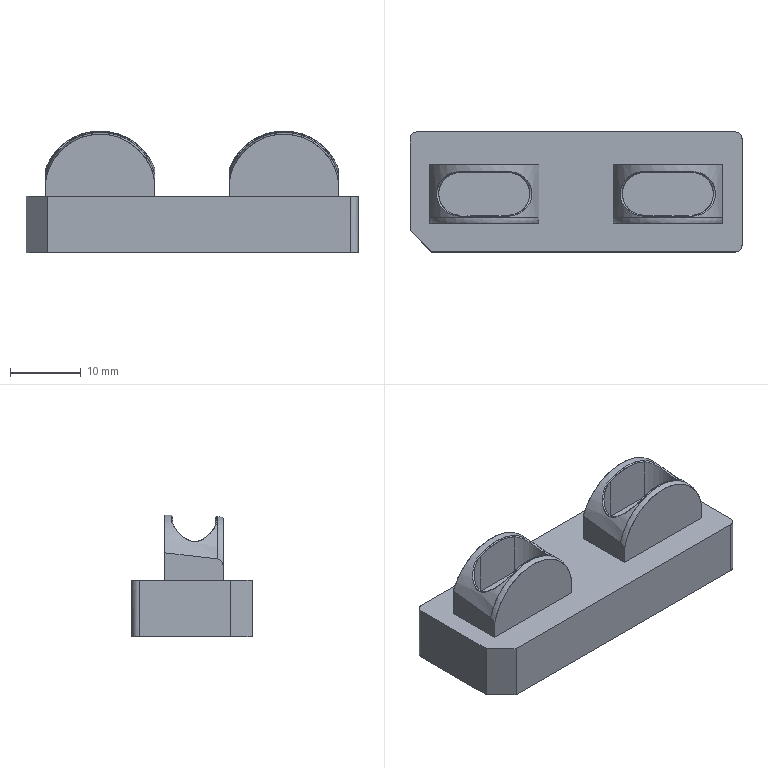NC program | PowerMill | posted with a generic post | part box 47 x 17 x 17.251 mm
Lines 19120 to 19835 of 158620:
N19217 M6
N19218 S22000 M03
N19219 G00 G90 X0.0 Y0.0
N19220 G43 Z10.798 H22
N19221
N19222 G05 P10000 R8
N19223 X21.9085 Y-5.0226
N19224 Z-6.8806
N19225 G01 Z-8.0806 F1200.0
N19226 X21.8959 Y-5.0352 Z-8.0493 F2000.0
N19227 X21.776 Y-5.0985 Z-7.6809
N19228 X21.7984 Y-5.0762 Z-7.7191
N19229 X21.8192 Y-5.0553 Z-7.7588
N19230 X21.8415 Y-5.033 Z-7.8048
N19231 X21.8681 Y-5.0064 Z-7.8637
N19232 X21.9 Y-4.9745 Z-7.9399
N19233 X21.9227 Y-4.9518 Z-7.9972
N19234 X21.9402 Y-4.9343 Z-8.0436
N19235 X21.9562 Y-4.9183 Z-8.0879
N19236 X21.9696 Y-4.9049 Z-8.1266
N19237 X22.0098 Y-4.8082 Z-8.1378
N19238 X22.0056 Y-4.8124 Z-8.1246
N19239 X21.9907 Y-4.8273 Z-8.0793
N19240 X21.9738 Y-4.8442 Z-8.0302
N19241 X21.9534 Y-4.8645 Z-7.9735
N19242 X21.9284 Y-4.8895 Z-7.9073
N19243 X21.8968 Y-4.9212 Z-7.8277
N19244 X21.8585 Y-4.9595 Z-7.7376
N19245 X21.8256 Y-4.9924 Z-7.6656
N19246 X21.7966 Y-5.0214 Z-7.6064
N19247 X21.7704 Y-5.0476 Z-7.5566
N19248 X21.7463 Y-5.0716 Z-7.5144
N19249 X21.7232 Y-5.0948 Z-7.4771
N19250 X21.6984 Y-5.1195 Z-7.4417
N19251 X21.6389 Y-5.1224 Z-7.2494
N19252 X21.6726 Y-5.0888 Z-7.2948
N19253 X21.7044 Y-5.0569 Z-7.3426
N19254 X21.7356 Y-5.0258 Z-7.3947
N19255 X21.7683 Y-4.9931 Z-7.4549
N19256 X21.8037 Y-4.9577 Z-7.5263
N19257 X21.8383 Y-4.923 Z-7.6003
N19258 X21.8719 Y-4.8895 Z-7.6747
N19259 X21.9129 Y-4.8485 Z-7.7716
N19260 X21.9529 Y-4.8085 Z-7.8737
N19261 X21.9897 Y-4.7717 Z-7.9758
N19262 X22.0228 Y-4.7385 Z-8.0758
N19263 X22.037 Y-4.7243 Z-8.1216
N19264 X22.0609 Y-4.6439 Z-8.1063
N19265 X22.0439 Y-4.6609 Z-8.0497
N19266 X22.0116 Y-4.6932 Z-7.9496
N19267 X21.9745 Y-4.7303 Z-7.8438
N19268 X21.9358 Y-4.769 Z-7.7414
N19269 X21.897 Y-4.8078 Z-7.6459
N19270 X21.8571 Y-4.8477 Z-7.5539
N19271 X21.8136 Y-4.8912 Z-7.46
N19272 X21.7702 Y-4.9346 Z-7.3732
N19273 X21.7462 Y-4.9586 Z-7.3279
N19274 X21.7218 Y-4.983 Z-7.2829
N19275 X21.6969 Y-5.0079 Z-7.2385
N19276 X21.6678 Y-5.037 Z-7.1906
N19277 X21.6402 Y-5.0646 Z-7.1495
N19278 X21.6114 Y-5.0934 Z-7.1105
N19279 X21.5813 Y-5.1235 Z-7.0731
N19280 X21.5247 Y-5.1236 Z-6.9091
N19281 X21.5585 Y-5.0898 Z-6.9483
N19282 X21.5926 Y-5.0557 Z-6.9927
N19283 X21.6276 Y-5.0206 Z-7.0437
N19284 X21.6648 Y-4.9834 Z-7.1031
N19285 X21.7063 Y-4.9419 Z-7.175
N19286 X21.7545 Y-4.8937 Z-7.263
N19287 X21.7917 Y-4.8565 Z-7.3347
N19288 X21.8271 Y-4.8211 Z-7.4081
N19289 X21.8612 Y-4.7871 Z-7.4829
N19290 X21.8979 Y-4.7504 Z-7.5683
N19291 X21.9396 Y-4.7086 Z-7.6715
N19292 X21.978 Y-4.6703 Z-7.7726
N19293 X22.0087 Y-4.6396 Z-7.8588
N19294 X22.0355 Y-4.6127 Z-7.9393
N19295 X22.0608 Y-4.5874 Z-8.0207
N19296 X22.0805 Y-4.5677 Z-8.0902
N19297 X22.0966 Y-4.495 Z-8.0754
N19298 X22.0885 Y-4.5031 Z-8.0396
N19299 X22.0746 Y-4.5171 Z-7.9886
N19300 X22.0622 Y-4.5295 Z-7.9464
N19301 X22.0417 Y-4.55 Z-7.8811
N19302 X22.0201 Y-4.5715 Z-7.8166
N19303 X21.9979 Y-4.5938 Z-7.7525
N19304 X21.9748 Y-4.6169 Z-7.6889
N19305 X21.9338 Y-4.6579 Z-7.5822
N19306 X21.8888 Y-4.7029 Z-7.4729
N19307 X21.8438 Y-4.7478 Z-7.3709
N19308 X21.8 Y-4.7917 Z-7.2781
N19309 X21.7575 Y-4.8342 Z-7.1942
N19310 X21.7077 Y-4.884 Z-7.1017
N19311 X21.662 Y-4.9296 Z-7.0222
N19312 X21.6188 Y-4.9729 Z-6.9524
N19313 X21.5758 Y-5.0159 Z-6.8886
N19314 X21.5376 Y-5.054 Z-6.8365
N19315 X21.5021 Y-5.0896 Z-6.7927
N19316 X21.4679 Y-5.1237 Z-6.7551
N19317 X21.4123 Y-5.1228 Z-6.6101
N19318 X21.4412 Y-5.0939 Z-6.6386
N19319 X21.4705 Y-5.0646 Z-6.6715
N19320 X21.503 Y-5.0321 Z-6.712
N19321 X21.5399 Y-4.9952 Z-6.7625
N19322 X21.5829 Y-4.9522 Z-6.8263
N19323 X21.6176 Y-4.9175 Z-6.8809
N19324 X21.6453 Y-4.8898 Z-6.9261
N19325 X21.6701 Y-4.865 Z-6.9673
N19326 X21.7179 Y-4.8172 Z-7.0514
N19327 X21.7653 Y-4.7698 Z-7.141
N19328 X21.8126 Y-4.7225 Z-7.237
N19329 X21.86 Y-4.6751 Z-7.3399
N19330 X21.9079 Y-4.6272 Z-7.451
N19331 X21.9454 Y-4.5897 Z-7.5432
N19332 X21.966 Y-4.5691 Z-7.5959
N19333 X21.9856 Y-4.5495 Z-7.6494
N19334 X22.0042 Y-4.5309 Z-7.7035
N19335 X22.0229 Y-4.5122 Z-7.7576
N19336 X22.0415 Y-4.4936 Z-7.8119
N19337 X22.0671 Y-4.468 Z-7.8937
N19338 X22.0889 Y-4.4462 Z-7.9723
N19339 X22.1072 Y-4.4279 Z-8.0482
N19340 X22.1079 Y-4.4272 Z-8.0517
N19341 X22.1147 Y-4.3639 Z-8.0167
N19342 X22.1118 Y-4.3667 Z-8.001
N19343 X22.1005 Y-4.378 Z-7.9478
N19344 X22.0853 Y-4.3933 Z-7.8892
N19345 X22.0647 Y-4.4138 Z-7.8208
N19346 X22.0341 Y-4.4445 Z-7.7261
N19347 X22.0009 Y-4.4776 Z-7.6281
N19348 X21.9614 Y-4.5171 Z-7.5202
N19349 X21.9196 Y-4.5589 Z-7.4145
N19350 X21.8759 Y-4.6026 Z-7.3121
N19351 X21.8305 Y-4.648 Z-7.2124
N19352 X21.7795 Y-4.699 Z-7.1066
N19353 X21.7297 Y-4.7488 Z-7.0096
N19354 X21.6804 Y-4.7981 Z-6.92
N19355 X21.6314 Y-4.8471 Z-6.8369
N19356 X21.5935 Y-4.885 Z-6.7766
N19357 X21.551 Y-4.9275 Z-6.7113
N19358 X21.5052 Y-4.9734 Z-6.6447
N19359 X21.4639 Y-5.0146 Z-6.5893
N19360 X21.4263 Y-5.0522 Z-6.5432
N19361 X21.3912 Y-5.0873 Z-6.5045
N19362 X21.3575 Y-5.121 Z-6.4717
N19363 X21.3027 Y-5.1193 Z-6.3407
N19364 X21.34 Y-5.0819 Z-6.3758
N19365 X21.3783 Y-5.0437 Z-6.4163
N19366 X21.4183 Y-5.0037 Z-6.4635
N19367 X21.4614 Y-4.9605 Z-6.5193
N19368 X21.4959 Y-4.9261 Z-6.5669
N19369 X21.5507 Y-4.8713 Z-6.647
N19370 X21.6048 Y-4.8172 Z-6.7317
N19371 X21.6583 Y-4.7637 Z-6.8213
N19372 X21.7112 Y-4.7107 Z-6.9162
N19373 X21.7638 Y-4.6582 Z-7.0167
N19374 X21.8161 Y-4.6059 Z-7.1233
N19375 X21.8682 Y-4.5537 Z-7.2364
N19376 X21.909 Y-4.513 Z-7.331
N19377 X21.9494 Y-4.4725 Z-7.4323
N19378 X21.9902 Y-4.4318 Z-7.5423
N19379 X22.0319 Y-4.39 Z-7.6631
N19380 X22.0633 Y-4.3586 Z-7.7594
N19381 X22.0856 Y-4.3363 Z-7.8337
N19382 X22.1027 Y-4.3193 Z-7.8985
N19383 X22.1157 Y-4.3062 Z-7.9578
N19384 X22.119 Y-4.3029 Z-7.975
N19385 X22.1223 Y-4.243 Z-7.9346
N19386 X22.116 Y-4.2494 Z-7.902
N19387 X22.1018 Y-4.2636 Z-7.8406
N19388 X22.0835 Y-4.2819 Z-7.7731
N19389 X22.0595 Y-4.3059 Z-7.6949
N19390 X22.0248 Y-4.3406 Z-7.5898
N19391 X21.9817 Y-4.3837 Z-7.4671
N19392 X21.9395 Y-4.4259 Z-7.3546
N19393 X21.8975 Y-4.4679 Z-7.2505
N19394 X21.8582 Y-4.5072 Z-7.1597
N19395 X21.8149 Y-4.5505 Z-7.0655
N19396 X21.7661 Y-4.5993 Z-6.9651
N19397 X21.713 Y-4.6524 Z-6.8626
N19398 X21.6603 Y-4.7051 Z-6.767
N19399 X21.6094 Y-4.756 Z-6.6803
N19400 X21.5605 Y-4.8048 Z-6.6025
N19401 X21.5103 Y-4.8551 Z-6.5278
N19402 X21.4566 Y-4.9088 Z-6.452
N19403 X21.4077 Y-4.9577 Z-6.3866
N19404 X21.3639 Y-5.0014 Z-6.3324
N19405 X21.3235 Y-5.0419 Z-6.2868
N19406 X21.2852 Y-5.0802 Z-6.248
N19407 X21.2485 Y-5.1169 Z-6.2151
N19408 X21.195 Y-5.1138 Z-6.0951
N19409 X21.2327 Y-5.0761 Z-6.1277
N19410 X21.2718 Y-5.037 Z-6.1661
N19411 X21.3135 Y-4.9953 Z-6.2116
N19412 X21.3599 Y-4.9489 Z-6.2669
N19413 X21.4167 Y-4.8922 Z-6.3392
N19414 X21.473 Y-4.8358 Z-6.416
N19415 X21.5291 Y-4.7798 Z-6.498
N19416 X21.581 Y-4.7279 Z-6.579
N19417 X21.6337 Y-4.6751 Z-6.6667
N19418 X21.6845 Y-4.6243 Z-6.7566
N19419 X21.7336 Y-4.5753 Z-6.8485
N19420 X21.7807 Y-4.5281 Z-6.9424
N19421 X21.8258 Y-4.483 Z-7.0383
N19422 X21.8754 Y-4.4334 Z-7.1502
N19423 X21.9229 Y-4.3859 Z-7.2651
N19424 X21.9682 Y-4.3406 Z-7.3824
N19425 X22.011 Y-4.2978 Z-7.5017
N19426 X22.0421 Y-4.2667 Z-7.5942
N19427 X22.0731 Y-4.2357 Z-7.6895
N19428 X22.0937 Y-4.2152 Z-7.7578
N19429 X22.1089 Y-4.1999 Z-7.8161
N19430 X22.1203 Y-4.1885 Z-7.869
N19431 X22.1249 Y-4.1839 Z-7.8952
N19432 X22.1263 Y-4.1259 Z-7.8568
N19433 X22.1201 Y-4.1322 Z-7.8218
N19434 X22.1113 Y-4.141 Z-7.7803
N19435 X22.101 Y-4.1512 Z-7.7394
N19436 X22.0863 Y-4.1659 Z-7.6889
N19437 X22.0723 Y-4.18 Z-7.6448
N19438 X22.0594 Y-4.1929 Z-7.6053
N19439 X22.0467 Y-4.2055 Z-7.5656
N19440 X22.0209 Y-4.2314 Z-7.4862
N19441 X21.9862 Y-4.2661 Z-7.3866
N19442 X21.946 Y-4.3062 Z-7.2791
N19443 X21.9038 Y-4.3484 Z-7.1729
N19444 X21.8637 Y-4.3886 Z-7.0774
N19445 X21.8219 Y-4.4303 Z-6.9834
N19446 X21.7709 Y-4.4814 Z-6.8752
N19447 X21.7185 Y-4.5337 Z-6.7712
N19448 X21.6648 Y-4.5874 Z-6.6713
N19449 X21.6099 Y-4.6424 Z-6.5754
N19450 X21.5536 Y-4.6986 Z-6.4835
N19451 X21.5294 Y-4.7229 Z-6.4457
N19452 X21.5047 Y-4.7476 Z-6.4085
N19453 X21.479 Y-4.7733 Z-6.3709
N19454 X21.4482 Y-4.804 Z-6.3274
N19455 X21.4107 Y-4.8416 Z-6.2762
N19456 X21.3627 Y-4.8896 Z-6.2136
N19457 X21.3114 Y-4.9409 Z-6.1505
N19458 X21.2692 Y-4.9831 Z-6.1018
N19459 X21.2329 Y-5.0194 Z-6.0627
N19460 X21.2009 Y-5.0514 Z-6.0306
N19461 X21.1707 Y-5.0815 Z-6.003
N19462 X21.1395 Y-5.1127 Z-5.9778
N19463 X21.0809 Y-5.1148 Z-5.8618
N19464 X21.1269 Y-5.0688 Z-5.8998
N19465 X21.1738 Y-5.0219 Z-5.943
N19466 X21.222 Y-4.9737 Z-5.992
N19467 X21.2719 Y-4.9238 Z-6.0476
N19468 X21.3244 Y-4.8713 Z-6.1109
N19469 X21.3808 Y-4.8149 Z-6.1837
N19470 X21.4421 Y-4.7536 Z-6.2671
N19471 X21.4956 Y-4.7001 Z-6.3446
N19472 X21.5435 Y-4.6522 Z-6.419
N19473 X21.5997 Y-4.596 Z-6.5116
N19474 X21.654 Y-4.5416 Z-6.6064
N19475 X21.7069 Y-4.4888 Z-6.7044
N19476 X21.7571 Y-4.4386 Z-6.8037
N19477 X21.8053 Y-4.3904 Z-6.9049
N19478 X21.8524 Y-4.3432 Z-7.0095
N19479 X21.8976 Y-4.2981 Z-7.1157
N19480 X21.9406 Y-4.2551 Z-7.2237
N19481 X21.9814 Y-4.2143 Z-7.3335
N19482 X22.0198 Y-4.1758 Z-7.4449
N19483 X22.0507 Y-4.1449 Z-7.5401
N19484 X22.0637 Y-4.132 Z-7.5803
N19485 X22.0773 Y-4.1183 Z-7.6224
N19486 X22.0933 Y-4.1024 Z-7.6733
N19487 X22.1067 Y-4.0889 Z-7.7216
N19488 X22.1166 Y-4.0791 Z-7.7634
N19489 X22.1249 Y-4.0708 Z-7.8058
N19490 X22.1277 Y-4.068 Z-7.8229
N19491 X22.1306 Y-4.0085 Z-7.8025
N19492 X22.1284 Y-4.0107 Z-7.7899
N19493 X22.1189 Y-4.0202 Z-7.7421
N19494 X22.1078 Y-4.0313 Z-7.695
N19495 X22.0952 Y-4.0439 Z-7.6486
N19496 X22.0805 Y-4.0586 Z-7.5996
N19497 X22.0662 Y-4.0729 Z-7.5541
N19498 X22.052 Y-4.0872 Z-7.5086
N19499 X22.0131 Y-4.126 Z-7.389
N19500 X21.9718 Y-4.1673 Z-7.271
N19501 X21.9277 Y-4.2114 Z-7.1536
N19502 X21.8816 Y-4.2575 Z-7.0393
N19503 X21.8352 Y-4.304 Z-6.9309
N19504 X21.7837 Y-4.3555 Z-6.818
N19505 X21.7305 Y-4.4086 Z-6.7087
N19506 X21.6758 Y-4.4633 Z-6.6031
N19507 X21.6195 Y-4.5196 Z-6.5012
N19508 X21.5618 Y-4.5774 Z-6.4029
N19509 X21.5025 Y-4.6366 Z-6.3083
N19510 X21.477 Y-4.6621 Z-6.2694
N19511 X21.451 Y-4.6882 Z-6.2312
N19512 X21.4244 Y-4.7147 Z-6.1936
N19513 X21.3937 Y-4.7454 Z-6.1516
N19514 X21.3572 Y-4.7819 Z-6.1031
N19515 X21.3123 Y-4.8269 Z-6.0458
N19516 X21.2549 Y-4.8842 Z-5.9764
N19517 X21.2036 Y-4.9355 Z-5.918
N19518 X21.1602 Y-4.9789 Z-5.8716
N19519 X21.1222 Y-5.0169 Z-5.8338
N19520 X21.0883 Y-5.0508 Z-5.8026
N19521 X21.0563 Y-5.0828 Z-5.7757
N19522 X21.0232 Y-5.1159 Z-5.7511
N19523 X20.966 Y-5.1166 Z-5.6438
N19524 X20.9675 Y-5.1151 Z-5.6449
N19525 X21.0063 Y-5.0763 Z-5.6736
N19526 X21.0439 Y-5.0386 Z-5.7049
N19527 X21.0838 Y-4.9987 Z-5.7412
N19528 X21.1276 Y-4.9549 Z-5.7844
N19529 X21.1765 Y-4.9061 Z-5.836
N19530 X21.2316 Y-4.851 Z-5.8984
N19531 X21.2932 Y-4.7893 Z-5.9729
N19532 X21.3456 Y-4.7369 Z-6.04
N19533 X21.3893 Y-4.6933 Z-6.0987
N19534 X21.4263 Y-4.6562 Z-6.1505
N19535 X21.4581 Y-4.6245 Z-6.1967
N19536 X21.4881 Y-4.5944 Z-6.2421
N19537 X21.5175 Y-4.5651 Z-6.2883
N19538 X21.5773 Y-4.5053 Z-6.3871
N19539 X21.6355 Y-4.447 Z-6.4893
N19540 X21.692 Y-4.3905 Z-6.5949
N19541 X21.7468 Y-4.3357 Z-6.7039
N19542 X21.7998 Y-4.2827 Z-6.8161
N19543 X21.851 Y-4.2316 Z-6.9316
N19544 X21.8951 Y-4.1875 Z-7.038
N19545 X21.9372 Y-4.1454 Z-7.146
N19546 X21.9787 Y-4.1039 Z-7.2589
N19547 X22.0204 Y-4.0621 Z-7.3793
N19548 X22.0571 Y-4.0255 Z-7.4912
N19549 X22.0918 Y-3.9908 Z-7.6043
N19550 X22.109 Y-3.9735 Z-7.6665
N19551 X22.1219 Y-3.9606 Z-7.722
N19552 X22.1313 Y-3.9512 Z-7.7732
N19553 X22.1327 Y-3.9498 Z-7.7824
N19554 X22.1341 Y-3.8919 Z-7.7628
N19555 X22.1315 Y-3.8945 Z-7.7441
N19556 X22.1238 Y-3.9022 Z-7.7023
N19557 X22.1122 Y-3.9138 Z-7.6542
N19558 X22.0946 Y-3.9314 Z-7.5903
N19559 X22.0741 Y-3.9519 Z-7.5202
N19560 X22.0419 Y-3.9841 Z-7.4167
N19561 X22.0081 Y-4.0179 Z-7.3143
N19562 X21.9723 Y-4.0537 Z-7.2116
N19563 X21.9355 Y-4.0905 Z-7.1112
N19564 X21.8971 Y-4.1289 Z-7.0121
N19565 X21.8465 Y-4.1795 Z-6.8895
N19566 X21.795 Y-4.231 Z-6.772
N19567 X21.7424 Y-4.2835 Z-6.6596
N19568 X21.6888 Y-4.3372 Z-6.5519
N19569 X21.6342 Y-4.3918 Z-6.4487
N19570 X21.5776 Y-4.4484 Z-6.3485
N19571 X21.5188 Y-4.5072 Z-6.2507
N19572 X21.4587 Y-4.5673 Z-6.1567
N19573 X21.3972 Y-4.6288 Z-6.0664
N19574 X21.3344 Y-4.6915 Z-5.9799
N19575 X21.2705 Y-4.7555 Z-5.8973
N19576 X21.2471 Y-4.7788 Z-5.8686
N19577 X21.2234 Y-4.8025 Z-5.8404
N19578 X21.1969 Y-4.829 Z-5.8099
N19579 X21.1645 Y-4.8614 Z-5.7738
N19580 X21.1231 Y-4.9029 Z-5.7293
N19581 X21.0688 Y-4.9572 Z-5.674
N19582 X21.0275 Y-4.9985 Z-5.6346
N19583 X20.9935 Y-5.0325 Z-5.6042
N19584 X20.9644 Y-5.0616 Z-5.58
N19585 X20.9373 Y-5.0887 Z-5.5596
N19586 X20.9094 Y-5.1166 Z-5.5412
N19587 X20.853 Y-5.1164 Z-5.4413
N19588 X20.8576 Y-5.1118 Z-5.4441
N19589 X20.8906 Y-5.0788 Z-5.4666
N19590 X20.9228 Y-5.0466 Z-5.4913
N19591 X20.9595 Y-5.0099 Z-5.5221
N19592 X21.0053 Y-4.9641 Z-5.5634
N19593 X21.0537 Y-4.9157 Z-5.61
N19594 X21.0898 Y-4.8796 Z-5.6466
N19595 X21.1194 Y-4.85 Z-5.6776
N19596 X21.1485 Y-4.8209 Z-5.7092
N19597 X21.2101 Y-4.7594 Z-5.7796
N19598 X21.2715 Y-4.6979 Z-5.8549
N19599 X21.3329 Y-4.6365 Z-5.9354
N19600 X21.3944 Y-4.575 Z-6.0214
N19601 X21.4553 Y-4.5141 Z-6.1122
N19602 X21.515 Y-4.4544 Z-6.2069
N19603 X21.5735 Y-4.3959 Z-6.3057
N19604 X21.6309 Y-4.3385 Z-6.4086
N19605 X21.6871 Y-4.2823 Z-6.5159
N19606 X21.7421 Y-4.2274 Z-6.6275
N19607 X21.7958 Y-4.1736 Z-6.7435
N19608 X21.8445 Y-4.1249 Z-6.8553
N19609 X21.8923 Y-4.0771 Z-6.9724
N19610 X21.9406 Y-4.0288 Z-7.0983
N19611 X21.9835 Y-3.9859 Z-7.2176
N19612 X22.0273 Y-3.9421 Z-7.3477
N19613 X22.0585 Y-3.9109 Z-7.4458
N19614 X22.0813 Y-3.8881 Z-7.5206
N19615 X22.1025 Y-3.8669 Z-7.5963
N19616 X22.1165 Y-3.8529 Z-7.6504
N19617 X22.1259 Y-3.8435 Z-7.6913
N19618 X22.1315 Y-3.8379 Z-7.7231
N19619 X22.1356 Y-3.8338 Z-7.7477
N19620 X22.1362 Y-3.7767 Z-7.7332
N19621 X22.1332 Y-3.7797 Z-7.7121
N19622 X22.1242 Y-3.7887 Z-7.6633
N19623 X22.1115 Y-3.8013 Z-7.6093
N19624 X22.0939 Y-3.8189 Z-7.5456
N19625 X22.0665 Y-3.8463 Z-7.454
N19626 X22.0523 Y-3.8606 Z-7.407
N19627 X22.0124 Y-3.9004 Z-7.2815
N19628 X21.9686 Y-3.9442 Z-7.1529
N19629 X21.9215 Y-3.9913 Z-7.0235
N19630 X21.8729 Y-4.0399 Z-6.8987
N19631 X21.8237 Y-4.0891 Z-6.78
N19632 X21.7743 Y-4.1385 Z-6.6679
N19633 X21.7206 Y-4.1922 Z-6.5532
N19634 X21.665 Y-4.2479 Z-6.4418
N19635 X21.6076 Y-4.3053 Z-6.3335
N19636 X21.5484 Y-4.3645 Z-6.2286
N19637 X21.4875 Y-4.4253 Z-6.1269
N19638 X21.425 Y-4.4879 Z-6.0286
N19639 X21.3765 Y-4.5363 Z-5.9568
N19640 X21.3265 Y-4.5863 Z-5.8871
N19641 X21.2753 Y-4.6376 Z-5.8193
N19642 X21.2154 Y-4.6974 Z-5.7438
N19643 X21.1618 Y-4.751 Z-5.6797
N19644 X21.107 Y-4.8059 Z-5.6178
N19645 X21.0831 Y-4.8298 Z-5.5921
N19646 X21.0588 Y-4.854 Z-5.5671
N19647 X21.0343 Y-4.8785 Z-5.5425
N19648 X21.0033 Y-4.9095 Z-5.5124
N19649 X20.9621 Y-4.9508 Z-5.4738
N19650 X20.9152 Y-4.9976 Z-5.4323
N19651 X20.8801 Y-5.0327 Z-5.403
N19652 X20.8515 Y-5.0614 Z-5.3807
N19653 X20.8248 Y-5.088 Z-5.3616
N19654 X20.7975 Y-5.1154 Z-5.3445
N19655 X20.7421 Y-5.1142 Z-5.2507
N19656 X20.7808 Y-5.0754 Z-5.275
N19657 X20.8186 Y-5.0377 Z-5.3018
N19658 X20.8581 Y-4.9981 Z-5.3328
N19659 X20.902 Y-4.9543 Z-5.3701
N19660 X20.9513 Y-4.905 Z-5.4151
N19661 X21.0078 Y-4.8485 Z-5.4704
N19662 X21.073 Y-4.7833 Z-5.5385
N19663 X21.1291 Y-4.7272 Z-5.6006
N19664 X21.1754 Y-4.6809 Z-5.6544
N19665 X21.2145 Y-4.6418 Z-5.7017
N19666 X21.248 Y-4.6083 Z-5.7438
N19667 X21.2793 Y-4.5769 Z-5.7845
N19668 X21.31 Y-4.5463 Z-5.8262
N19669 X21.3745 Y-4.4817 Z-5.9182
N19670 X21.4376 Y-4.4186 Z-6.0139
N19671 X21.4992 Y-4.3571 Z-6.1131
N19672 X21.5592 Y-4.2971 Z-6.2158
N19673 X21.6176 Y-4.2387 Z-6.3219
N19674 X21.6743 Y-4.182 Z-6.4315
N19675 X21.7262 Y-4.13 Z-6.5382
N19676 X21.7765 Y-4.0798 Z-6.6478
N19677 X21.8251 Y-4.0312 Z-6.76
N19678 X21.8765 Y-3.9798 Z-6.8857
N19679 X21.9207 Y-3.9356 Z-7.0004
N19680 X21.9628 Y-3.8935 Z-7.1166
N19681 X21.9966 Y-3.8597 Z-7.2158
N19682 X22.0292 Y-3.8271 Z-7.3159
N19683 X22.0603 Y-3.796 Z-7.4169
N19684 X22.0806 Y-3.7757 Z-7.4839
N19685 X22.0958 Y-3.7605 Z-7.538
N19686 X22.1074 Y-3.7489 Z-7.5833
N19687 X22.1183 Y-3.738 Z-7.6289
N19688 X22.1283 Y-3.728 Z-7.6749
N19689 X22.1363 Y-3.7199 Z-7.7187
N19690 X22.136 Y-3.6637 Z-7.7068
N19691 X22.1293 Y-3.6704 Z-7.6684
N19692 X22.1203 Y-3.6794 Z-7.6263
N19693 X22.1097 Y-3.69 Z-7.5818
N19694 X22.0953 Y-3.7044 Z-7.5266
N19695 X22.0739 Y-3.7258 Z-7.4501
N19696 X22.0552 Y-3.7445 Z-7.3871
N19697 X22.0406 Y-3.7591 Z-7.3393
N19698 X22.0278 Y-3.7719 Z-7.2981
N19699 X21.9879 Y-3.8118 Z-7.1749
N19700 X21.9458 Y-3.8539 Z-7.0523
N19701 X21.9 Y-3.8997 Z-6.9269
N19702 X21.8521 Y-3.9476 Z-6.804
N19703 X21.8036 Y-3.9961 Z-6.6872
N19704 X21.7528 Y-4.0469 Z-6.5723
N19705 X21.7 Y-4.0997 Z-6.4593
N19706 X21.6485 Y-4.1512 Z-6.355
N19707 X21.5916 Y-4.2081 Z-6.2461
N19708 X21.5335 Y-4.2662 Z-6.1414
N19709 X21.4742 Y-4.3255 Z-6.041
N19710 X21.4137 Y-4.386 Z-5.9446
N19711 X21.352 Y-4.4477 Z-5.8519
N19712 X21.2883 Y-4.5115 Z-5.7621
N19713 X21.2264 Y-4.5733 Z-5.68
N19714 X21.1632 Y-4.6365 Z-5.6008
N19715 X21.1002 Y-4.6995 Z-5.5267
N19716 X21.038 Y-4.7617 Z-5.4585
N19717 X20.9757 Y-4.824 Z-5.3948
N19718 X20.9118 Y-4.8879 Z-5.3344
N19719 X20.8566 Y-4.9432 Z-5.2844
N19720 X20.8064 Y-4.9933 Z-5.2414
N19721 X20.7635 Y-5.0362 Z-5.2081
N19722 X20.7243 Y-5.0754 Z-5.1814
N19723 X20.6871 Y-5.1126 Z-5.16
N19724 X20.6324 Y-5.1107 Z-5.0711
N19725 X20.6697 Y-5.0735 Z-5.0927
N19726 X20.706 Y-5.0371 Z-5.1168
N19727 X20.7443 Y-4.9989 Z-5.1448
N19728 X20.7876 Y-4.9555 Z-5.1792
N19729 X20.8378 Y-4.9053 Z-5.2221
N19730 X20.898 Y-4.8451 Z-5.2771
N19731 X20.9571 Y-4.786 Z-5.3346
N19732 X21.0042 Y-4.7389 Z-5.3828
N19733 X21.0432 Y-4.6999 Z-5.4243
N19734 X21.0762 Y-4.667 Z-5.4606
N19735 X21.1076 Y-4.6355 Z-5.4965
N19736 X21.1385 Y-4.6046 Z-5.5332
N19737 X21.2049 Y-4.5382 Z-5.6164
N19738 X21.2703 Y-4.4728 Z-5.7036
N19739 X21.3347 Y-4.4085 Z-5.7948
N19740 X21.3979 Y-4.3452 Z-5.8901
N19741 X21.4599 Y-4.2832 Z-5.9894
N19742 X21.5207 Y-4.2224 Z-6.0927
N19743 X21.5802 Y-4.1629 Z-6.2
N19744 X21.633 Y-4.1101 Z-6.3009
N19745 X21.6881 Y-4.055 Z-6.4124
N19746 X21.7409 Y-4.0022 Z-6.5261
N19747 X21.7937 Y-3.9494 Z-6.6469
N19748 X21.8468 Y-3.8964 Z-6.7755
N19749 X21.8985 Y-3.8446 Z-6.9081
N19750 X21.9333 Y-3.8098 Z-7.0017
N19751 X21.9685 Y-3.7746 Z-7.1034
N19752 X22.0103 Y-3.7329 Z-7.232
N19753 X22.029 Y-3.7142 Z-7.291
N19754 X22.04 Y-3.7031 Z-7.3269
N19755 X22.0509 Y-3.6923 Z-7.363
N19756 X22.0622 Y-3.6809 Z-7.4011
N19757 X22.0728 Y-3.6703 Z-7.4373
N19758 X22.0833 Y-3.6599 Z-7.4736
N19759 X22.0935 Y-3.6497 Z-7.5101
N19760 X22.103 Y-3.6402 Z-7.5469
N19761 X22.1199 Y-3.6233 Z-7.6161
N19762 X22.1315 Y-3.6117 Z-7.6719
N19763 X22.1357 Y-3.6075 Z-7.6959
N19764 X22.1351 Y-3.5515 Z-7.6851
N19765 X22.132 Y-3.5545 Z-7.6658
N19766 X22.1267 Y-3.5599 Z-7.6364
N19767 X22.1137 Y-3.5729 Z-7.5796
N19768 X22.0997 Y-3.5869 Z-7.5242
N19769 X22.0836 Y-3.6029 Z-7.4674
N19770 X22.0678 Y-3.6187 Z-7.413
N19771 X22.0461 Y-3.6404 Z-7.3394
N19772 X22.0238 Y-3.6627 Z-7.2662
N19773 X22.0011 Y-3.6855 Z-7.1933
N19774 X21.9662 Y-3.7204 Z-7.0862
N19775 X21.9204 Y-3.7662 Z-6.9543
N19776 X21.8714 Y-3.8152 Z-6.8222
N19777 X21.8204 Y-3.8661 Z-6.6932
N19778 X21.7676 Y-3.9189 Z-6.5675
N19779 X21.7132 Y-3.9734 Z-6.4457
N19780 X21.6574 Y-4.0292 Z-6.3279
N19781 X21.6002 Y-4.0863 Z-6.2144
N19782 X21.542 Y-4.1446 Z-6.1055
N19783 X21.4827 Y-4.2038 Z-6.001
N19784 X21.4221 Y-4.2645 Z-5.9003
N19785 X21.3588 Y-4.3278 Z-5.8014
N19786 X21.2942 Y-4.3924 Z-5.7062
N19787 X21.2283 Y-4.4583 Z-5.6148
N19788 X21.1612 Y-4.5254 Z-5.5272
N19789 X21.0928 Y-4.5937 Z-5.4434
N19790 X21.0614 Y-4.6252 Z-5.4067
N19791 X21.0294 Y-4.6572 Z-5.3709
N19792 X20.9953 Y-4.6913 Z-5.3341
N19793 X20.9549 Y-4.7317 Z-5.2921
N19794 X20.906 Y-4.7806 Z-5.2435
N19795 X20.8446 Y-4.842 Z-5.1854
N19796 X20.7844 Y-4.9022 Z-5.132
N19797 X20.734 Y-4.9526 Z-5.0903
N19798 X20.6904 Y-4.9962 Z-5.0567
N19799 X20.6518 Y-5.0347 Z-5.0293
N19800 X20.6149 Y-5.0716 Z-5.0055
N19801 X20.5772 Y-5.1094 Z-4.9843
N19802 X20.5197 Y-5.1103 Z-4.8984
N19803 X20.5578 Y-5.0722 Z-4.9191
N19804 X20.5951 Y-5.0349 Z-4.9423
N19805 X20.634 Y-4.996 Z-4.9691
N19806 X20.6781 Y-4.9519 Z-5.002
N19807 X20.7291 Y-4.9009 Z-5.043
N19808 X20.7901 Y-4.8399 Z-5.0955
N19809 X20.8522 Y-4.7778 Z-5.1525
N19810 X20.9016 Y-4.7284 Z-5.2002
N19811 X20.9424 Y-4.6876 Z-5.2414
N19812 X20.9769 Y-4.6531 Z-5.2775
N19813 X21.0095 Y-4.6205 Z-5.3128
N19814 X21.0414 Y-4.5886 Z-5.349
N19815 X21.1095 Y-4.5205 Z-5.4299
N19816 X21.1765 Y-4.4535 Z-5.5148
N19817 X21.2425 Y-4.3875 Z-5.6037
N19818 X21.3073 Y-4.3227 Z-5.6966
N19819 X21.3711 Y-4.2589 Z-5.7936
N19820 X21.4337 Y-4.1963 Z-5.8947
N19821 X21.4951 Y-4.1349 Z-5.9999
N19822 X21.5553 Y-4.0747 Z-6.1091
N19823 X21.6141 Y-4.0159 Z-6.2221
N19824 X21.6709 Y-3.9591 Z-6.3379
N19825 X21.7256 Y-3.9044 Z-6.4565
N19826 X21.7782 Y-3.8518 Z-6.5777
N19827 X21.8264 Y-3.8036 Z-6.6954
N19828 X21.8728 Y-3.7572 Z-6.8145
N19829 X21.9172 Y-3.7128 Z-6.9351
N19830 X21.9594 Y-3.6706 Z-7.0572
N19831 X21.9971 Y-3.6329 Z-7.1733
N19832 X22.0427 Y-3.5873 Z-7.3185
N19833 X22.0742 Y-3.5558 Z-7.4241
N19834 X22.0974 Y-3.5326 Z-7.5092
N19835 X22.1096 Y-3.5204 Z-7.5566
N19836 X22.1236 Y-3.5064 Z-7.6157
N19837 X22.1329 Y-3.4971 Z-7.6642
N19838 X22.1346 Y-3.4954 Z-7.6748
N19839 X22.1345 Y-3.439 Z-7.6656
N19840 X22.1284 Y-3.445 Z-7.6293
N19841 X22.1222 Y-3.4512 Z-7.5999
N19842 X22.1083 Y-3.4651 Z-7.5436
N19843 X22.0863 Y-3.4871 Z-7.4611
N19844 X22.0626 Y-3.5109 Z-7.3796
N19845 X22.0373 Y-3.5361 Z-7.2969
N19846 X21.9861 Y-3.5873 Z-7.1343
N19847 X21.9366 Y-3.6369 Z-6.9855
N19848 X21.8863 Y-3.6871 Z-6.8435
N19849 X21.8353 Y-3.7381 Z-6.7079
N19850 X21.7835 Y-3.79 Z-6.5781
N19851 X21.7307 Y-3.8428 Z-6.4537
N19852 X21.6769 Y-3.8966 Z-6.3345
N19853 X21.622 Y-3.9514 Z-6.2201
N19854 X21.5651 Y-4.0084 Z-6.108
N19855 X21.506 Y-4.0675 Z-5.9979
N19856 X21.4462 Y-4.1272 Z-5.893
N19857 X21.3836 Y-4.1898 Z-5.7893
N19858 X21.3196 Y-4.2538 Z-5.6894
N19859 X21.2544 Y-4.3191 Z-5.5933
N19860 X21.1879 Y-4.3856 Z-5.5011
N19861 X21.1202 Y-4.4533 Z-5.4127
N19862 X21.0513 Y-4.5221 Z-5.3282
N19863 X20.9814 Y-4.5921 Z-5.2475
N19864 X20.9499 Y-4.6235 Z-5.2132
N19865 X20.918 Y-4.6554 Z-5.1797
N19866 X20.8829 Y-4.6906 Z-5.1442
N19867 X20.8412 Y-4.7323 Z-5.1036
N19868 X20.7904 Y-4.783 Z-5.0563
N19869 X20.7259 Y-4.8475 Z-4.9993
N19870 X20.6665 Y-4.9069 Z-4.9502
N19871 X20.617 Y-4.9565 Z-4.9119
N19872 X20.5742 Y-4.9993 Z-4.8811
N19873 X20.5364 Y-5.037 Z-4.8561
N19874 X20.5 Y-5.0734 Z-4.8344
N19875 X20.4628 Y-5.1106 Z-4.8152
N19876 X20.4062 Y-5.1107 Z-4.7334
N19877 X20.4095 Y-5.1074 Z-4.7349
N19878 X20.4468 Y-5.0701 Z-4.7537
N19879 X20.4833 Y-5.0336 Z-4.775
N19880 X20.5216 Y-4.9953 Z-4.7998
N19881 X20.5651 Y-4.9517 Z-4.8304
N19882 X20.6156 Y-4.9012 Z-4.8685
N19883 X20.6763 Y-4.8405 Z-4.9177
N19884 X20.7406 Y-4.7763 Z-4.9733
N19885 X20.7913 Y-4.7256 Z-5.0196
N19886 X20.833 Y-4.6839 Z-5.0593
N19887 X20.8682 Y-4.6486 Z-5.0941
N19888 X20.9004 Y-4.6164 Z-5.127
N19889 X20.9321 Y-4.5847 Z-5.1609
N19890 X21.0046 Y-4.5123 Z-5.2423
N19891 X21.0748 Y-4.4421 Z-5.3263
N19892 X21.1427 Y-4.3741 Z-5.4128
N19893 X21.2084 Y-4.3085 Z-5.5017
N19894 X21.2719 Y-4.245 Z-5.5931
N19895 X21.3371 Y-4.1798 Z-5.6926
N19896 X21.4008 Y-4.116 Z-5.7958
N19897 X21.4632 Y-4.0537 Z-5.9027
N19898 X21.5241 Y-3.9928 Z-6.0134
N19899 X21.5835 Y-3.9334 Z-6.1278
N19900 X21.6413 Y-3.8756 Z-6.246
N19901 X21.6976 Y-3.8193 Z-6.368
N19902 X21.7522 Y-3.7646 Z-6.4936
N19903 X21.8052 Y-3.7117 Z-6.623
N19904 X21.8584 Y-3.6585 Z-6.7606
N19905 X21.911 Y-3.6059 Z-6.9049
N19906 X21.9631 Y-3.5537 Z-7.0565
N19907 X22.0147 Y-3.5021 Z-7.2155
N19908 X22.0586 Y-3.4582 Z-7.3589
N19909 X22.0778 Y-3.4391 Z-7.4239
N19910 X22.096 Y-3.4209 Z-7.4887
N19911 X22.1114 Y-3.4055 Z-7.5481
N19912 X22.1256 Y-3.3913 Z-7.6082
N19913 X22.1306 Y-3.3863 Z-7.6339
N19914 X22.1342 Y-3.3827 Z-7.6564
N19915 X22.1341 Y-3.3262 Z-7.6471
N19916 X22.1314 Y-3.3289 Z-7.6306
N19917 X22.1213 Y-3.339 Z-7.5804
N19918 X22.1066 Y-3.3537 Z-7.5202
N19919 X22.0942 Y-3.3661 Z-7.4736
N19920 X22.0749 Y-3.3854 Z-7.4069
N19921 X22.0549 Y-3.4054 Z-7.3405
N19922 X22.0347 Y-3.4256 Z-7.2742
N19923 X22.0075 Y-3.4527 Z-7.1865
N19924 X21.9654 Y-3.4949 Z-7.0573
N19925 X21.9214 Y-3.5389 Z-6.9293
N19926 X21.8713 Y-3.589 Z-6.7904
N19927 X21.8239 Y-3.6364 Z-6.6648
N19928 X21.7749 Y-3.6854 Z-6.5405
N19929 X21.7238 Y-3.7365 Z-6.4178
N19930 X21.669 Y-3.7913 Z-6.2936
N19931 X21.6123 Y-3.848 Z-6.1725
N19932 X21.5536 Y-3.9067 Z-6.0545